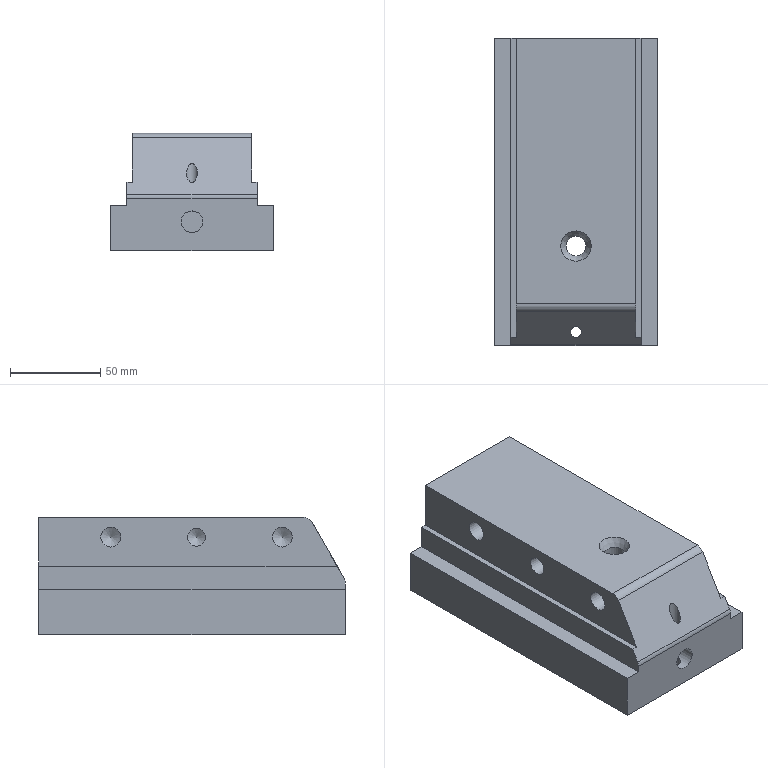Part | NX | features solid 2 | 1 solid | 47 faces | box 90 x 170 x 65 mm | volume 622794 mm3 | plane 25 | cylinder 16 | cone 6 | commonest cylinder face diameters 11 x5 4 x4 10 x3 6 x2 12 x2
STEP:
#1=CARTESIAN_POINT('',(-3.,607.5,-122.196));
#2=VERTEX_POINT('',#1);
#3=CARTESIAN_POINT('',(-2.354,609.851,-122.626));
#4=CARTESIAN_POINT('',(-3.324,607.499,-121.981));
#5=CARTESIAN_POINT('',(-2.352,605.153,-122.625));
#6=CARTESIAN_POINT('',(-0.009342,604.174,-123.187));
#7=CARTESIAN_POINT('',(2.352,605.151,-122.627));
#8=CARTESIAN_POINT('',(3.323,607.488,-121.981));
#9=CARTESIAN_POINT('',(2.356,609.847,-122.624));
#10=CARTESIAN_POINT('',(0.009754,610.826,-123.187));
#11=CARTESIAN_POINT('',(-2.354,609.851,-122.626));
#12=CARTESIAN_POINT('',(-3.324,607.499,-121.981));
#13=CARTESIAN_POINT('',(-2.352,605.153,-122.625));
#14=B_SPLINE_CURVE_WITH_KNOTS('',3,(#3,#4,#5,#6,#7,#8,#9,#10,#11,#12,#13),.UNSPECIFIED.,.T.,.F.,(1,1,1,1,1,1,1,1,1,1,1,1,1,1,1),(-0.00715,-0.004767,-0.002383,0.,0.002383,0.004767,0.00715,0.009533,0.01192,0.0143,0.01668,0.01907,0.02145,0.02383,0.02622),.UNSPECIFIED.);
#15=EDGE_CURVE('',#2,#2,#14,.T.);
#16=ORIENTED_EDGE('',*,*,#15,.T.);
#17=EDGE_LOOP('',(#16));
#18=FACE_BOUND('',#17,.T.);
#19=CARTESIAN_POINT('',(-3.,607.5,-133.));
#20=VERTEX_POINT('',#19);
#21=CARTESIAN_POINT('',(0.,607.5,-133.));
#22=DIRECTION('',(0.,0.,1.));
#23=DIRECTION('',(-1.,0.,0.));
#24=AXIS2_PLACEMENT_3D('',#21,#22,#23);
#25=CIRCLE('',#24,3.);
#26=EDGE_CURVE('',#20,#20,#25,.T.);
#27=ORIENTED_EDGE('',*,*,#26,.F.);
#28=EDGE_LOOP('',(#27));
#29=FACE_BOUND('',#28,.T.);
#30=CARTESIAN_POINT('',(0.,607.5,-133.));
#31=DIRECTION('',(0.,0.,1.));
#32=DIRECTION('',(-1.,0.,0.));
#33=AXIS2_PLACEMENT_3D('',#30,#31,#32);
#34=CYLINDRICAL_SURFACE('',#33,3.);
#35=ADVANCED_FACE('',(#18,#29),#34,.F.);
#36=CARTESIAN_POINT('',(33.,604.619,-95.));
#37=VERTEX_POINT('',#36);
#38=CARTESIAN_POINT('',(33.,770.,-95.));
#39=VERTEX_POINT('',#38);
#40=CARTESIAN_POINT('',(33.,600.,-95.));
#41=DIRECTION('',(0.,1.,0.));
#42=VECTOR('',#41,1000.);
#43=LINE('',#40,#42);
#44=EDGE_CURVE('',#37,#39,#43,.T.);
#45=ORIENTED_EDGE('',*,*,#44,.F.);
#46=CARTESIAN_POINT('',(36.,604.619,-95.));
#47=VERTEX_POINT('',#46);
#48=CARTESIAN_POINT('',(33.,604.619,-95.));
#49=DIRECTION('',(1.,0.,0.));
#50=VECTOR('',#49,1000.);
#51=LINE('',#48,#50);
#52=EDGE_CURVE('',#37,#47,#51,.T.);
#53=ORIENTED_EDGE('',*,*,#52,.T.);
#54=CARTESIAN_POINT('',(36.,770.,-95.));
#55=VERTEX_POINT('',#54);
#56=CARTESIAN_POINT('',(36.,600.,-95.));
#57=DIRECTION('',(0.,1.,0.));
#58=VECTOR('',#57,1000.);
#59=LINE('',#56,#58);
#60=EDGE_CURVE('',#47,#55,#59,.T.);
#61=ORIENTED_EDGE('',*,*,#60,.T.);
#62=CARTESIAN_POINT('',(33.,770.,-95.));
#63=DIRECTION('',(1.,0.,0.));
#64=VECTOR('',#63,1000.);
#65=LINE('',#62,#64);
#66=EDGE_CURVE('',#39,#55,#65,.T.);
#67=ORIENTED_EDGE('',*,*,#66,.F.);
#68=EDGE_LOOP('',(#45,#53,#61,#67));
#69=FACE_BOUND('',#68,.T.);
#70=CARTESIAN_POINT('',(33.,600.,-95.));
#71=DIRECTION('',(0.,0.,1.));
#72=DIRECTION('',(0.,-1.,0.));
#73=AXIS2_PLACEMENT_3D('',#70,#71,#72);
#74=PLANE('',#73);
#75=ADVANCED_FACE('',(#69),#74,.T.);
#76=CARTESIAN_POINT('',(36.,600.67,-101.84));
#77=VERTEX_POINT('',#76);
#78=CARTESIAN_POINT('',(36.,603.464,-97.));
#79=DIRECTION('',(0.,-0.5,-0.866));
#80=VECTOR('',#79,1000.);
#81=LINE('',#78,#80);
#82=EDGE_CURVE('',#47,#77,#81,.T.);
#83=ORIENTED_EDGE('',*,*,#82,.T.);
#84=CARTESIAN_POINT('',(36.,600.,-104.34));
#85=VERTEX_POINT('',#84);
#86=CARTESIAN_POINT('',(36.,605.,-104.34));
#87=DIRECTION('',(1.,0.,0.));
#88=DIRECTION('',(0.,0.,1.));
#89=AXIS2_PLACEMENT_3D('',#86,#87,#88);
#90=CIRCLE('',#89,5.);
#91=EDGE_CURVE('',#77,#85,#90,.T.);
#92=ORIENTED_EDGE('',*,*,#91,.T.);
#93=CARTESIAN_POINT('',(36.,600.,-108.));
#94=VERTEX_POINT('',#93);
#95=CARTESIAN_POINT('',(36.,600.,-95.));
#96=DIRECTION('',(0.,0.,-1.));
#97=VECTOR('',#96,1000.);
#98=LINE('',#95,#97);
#99=EDGE_CURVE('',#85,#94,#98,.T.);
#100=ORIENTED_EDGE('',*,*,#99,.T.);
#101=CARTESIAN_POINT('',(36.,770.,-108.));
#102=VERTEX_POINT('',#101);
#103=CARTESIAN_POINT('',(36.,600.,-108.));
#104=DIRECTION('',(0.,1.,0.));
#105=VECTOR('',#104,1000.);
#106=LINE('',#103,#105);
#107=EDGE_CURVE('',#94,#102,#106,.T.);
#108=ORIENTED_EDGE('',*,*,#107,.T.);
#109=CARTESIAN_POINT('',(36.,770.,-95.));
#110=DIRECTION('',(0.,0.,-1.));
#111=VECTOR('',#110,1000.);
#112=LINE('',#109,#111);
#113=EDGE_CURVE('',#55,#102,#112,.T.);
#114=ORIENTED_EDGE('',*,*,#113,.F.);
#115=ORIENTED_EDGE('',*,*,#60,.F.);
#116=EDGE_LOOP('',(#83,#92,#100,#108,#114,#115));
#117=FACE_BOUND('',#116,.T.);
#118=CARTESIAN_POINT('',(36.,600.,-95.));
#119=DIRECTION('',(1.,0.,0.));
#120=DIRECTION('',(0.,0.,1.));
#121=AXIS2_PLACEMENT_3D('',#118,#119,#120);
#122=PLANE('',#121);
#123=ADVANCED_FACE('',(#117),#122,.T.);
#124=CARTESIAN_POINT('',(45.,770.,-108.));
#125=VERTEX_POINT('',#124);
#126=CARTESIAN_POINT('',(36.,770.,-108.));
#127=DIRECTION('',(1.,0.,0.));
#128=VECTOR('',#127,1000.);
#129=LINE('',#126,#128);
#130=EDGE_CURVE('',#102,#125,#129,.T.);
#131=ORIENTED_EDGE('',*,*,#130,.F.);
#132=ORIENTED_EDGE('',*,*,#107,.F.);
#133=CARTESIAN_POINT('',(45.,600.,-108.));
#134=VERTEX_POINT('',#133);
#135=CARTESIAN_POINT('',(36.,600.,-108.));
#136=DIRECTION('',(1.,0.,0.));
#137=VECTOR('',#136,1000.);
#138=LINE('',#135,#137);
#139=EDGE_CURVE('',#94,#134,#138,.T.);
#140=ORIENTED_EDGE('',*,*,#139,.T.);
#141=CARTESIAN_POINT('',(45.,600.,-108.));
#142=DIRECTION('',(0.,1.,0.));
#143=VECTOR('',#142,1000.);
#144=LINE('',#141,#143);
#145=EDGE_CURVE('',#134,#125,#144,.T.);
#146=ORIENTED_EDGE('',*,*,#145,.T.);
#147=EDGE_LOOP('',(#131,#132,#140,#146));
#148=FACE_BOUND('',#147,.T.);
#149=CARTESIAN_POINT('',(36.,600.,-108.));
#150=DIRECTION('',(0.,0.,1.));
#151=DIRECTION('',(0.,-1.,0.));
#152=AXIS2_PLACEMENT_3D('',#149,#150,#151);
#153=PLANE('',#152);
#154=ADVANCED_FACE('',(#148),#153,.T.);
#155=CARTESIAN_POINT('',(45.,770.,-133.));
#156=VERTEX_POINT('',#155);
#157=CARTESIAN_POINT('',(45.,770.,-108.));
#158=DIRECTION('',(0.,0.,-1.));
#159=VECTOR('',#158,1000.);
#160=LINE('',#157,#159);
#161=EDGE_CURVE('',#125,#156,#160,.T.);
#162=ORIENTED_EDGE('',*,*,#161,.F.);
#163=ORIENTED_EDGE('',*,*,#145,.F.);
#164=CARTESIAN_POINT('',(45.,600.,-133.));
#165=VERTEX_POINT('',#164);
#166=CARTESIAN_POINT('',(45.,600.,-108.));
#167=DIRECTION('',(0.,0.,-1.));
#168=VECTOR('',#167,1000.);
#169=LINE('',#166,#168);
#170=EDGE_CURVE('',#134,#165,#169,.T.);
#171=ORIENTED_EDGE('',*,*,#170,.T.);
#172=CARTESIAN_POINT('',(45.,600.,-133.));
#173=DIRECTION('',(0.,1.,0.));
#174=VECTOR('',#173,1000.);
#175=LINE('',#172,#174);
#176=EDGE_CURVE('',#165,#156,#175,.T.);
#177=ORIENTED_EDGE('',*,*,#176,.T.);
#178=EDGE_LOOP('',(#162,#163,#171,#177));
#179=FACE_BOUND('',#178,.T.);
#180=CARTESIAN_POINT('',(45.,600.,-108.));
#181=DIRECTION('',(1.,0.,0.));
#182=DIRECTION('',(0.,0.,1.));
#183=AXIS2_PLACEMENT_3D('',#180,#181,#182);
#184=PLANE('',#183);
#185=ADVANCED_FACE('',(#179),#184,.T.);
#186=CARTESIAN_POINT('',(18.,615.,-133.));
#187=VERTEX_POINT('',#186);
#188=CARTESIAN_POINT('',(-18.,615.,-133.));
#189=VERTEX_POINT('',#188);
#190=CARTESIAN_POINT('',(20.,615.,-133.));
#191=DIRECTION('',(-1.,0.,0.));
#192=VECTOR('',#191,1000.);
#193=LINE('',#190,#192);
#194=EDGE_CURVE('',#187,#189,#193,.T.);
#195=ORIENTED_EDGE('',*,*,#194,.F.);
#196=CARTESIAN_POINT('',(20.,617.,-133.));
#197=VERTEX_POINT('',#196);
#198=CARTESIAN_POINT('',(18.,617.,-133.));
#199=DIRECTION('',(0.,0.,-1.));
#200=DIRECTION('',(0.,1.,0.));
#201=AXIS2_PLACEMENT_3D('',#198,#199,#200);
#202=CIRCLE('',#201,2.);
#203=EDGE_CURVE('',#187,#197,#202,.F.);
#204=ORIENTED_EDGE('',*,*,#203,.T.);
#205=CARTESIAN_POINT('',(20.,753.,-133.));
#206=VERTEX_POINT('',#205);
#207=CARTESIAN_POINT('',(20.,615.,-133.));
#208=DIRECTION('',(0.,1.,0.));
#209=VECTOR('',#208,1000.);
#210=LINE('',#207,#209);
#211=EDGE_CURVE('',#197,#206,#210,.T.);
#212=ORIENTED_EDGE('',*,*,#211,.T.);
#213=CARTESIAN_POINT('',(18.,755.,-133.));
#214=VERTEX_POINT('',#213);
#215=CARTESIAN_POINT('',(18.,753.,-133.));
#216=DIRECTION('',(0.,0.,-1.));
#217=DIRECTION('',(0.,1.,0.));
#218=AXIS2_PLACEMENT_3D('',#215,#216,#217);
#219=CIRCLE('',#218,2.);
#220=EDGE_CURVE('',#206,#214,#219,.F.);
#221=ORIENTED_EDGE('',*,*,#220,.T.);
#222=CARTESIAN_POINT('',(-18.,755.,-133.));
#223=VERTEX_POINT('',#222);
#224=CARTESIAN_POINT('',(20.,755.,-133.));
#225=DIRECTION('',(-1.,0.,0.));
#226=VECTOR('',#225,1000.);
#227=LINE('',#224,#226);
#228=EDGE_CURVE('',#214,#223,#227,.T.);
#229=ORIENTED_EDGE('',*,*,#228,.T.);
#230=CARTESIAN_POINT('',(-20.,753.,-133.));
#231=VERTEX_POINT('',#230);
#232=CARTESIAN_POINT('',(-18.,753.,-133.));
#233=DIRECTION('',(0.,0.,-1.));
#234=DIRECTION('',(0.,1.,0.));
#235=AXIS2_PLACEMENT_3D('',#232,#233,#234);
#236=CIRCLE('',#235,2.);
#237=EDGE_CURVE('',#223,#231,#236,.F.);
#238=ORIENTED_EDGE('',*,*,#237,.T.);
#239=CARTESIAN_POINT('',(-20.,617.,-133.));
#240=VERTEX_POINT('',#239);
#241=CARTESIAN_POINT('',(-20.,615.,-133.));
#242=DIRECTION('',(0.,1.,0.));
#243=VECTOR('',#242,1000.);
#244=LINE('',#241,#243);
#245=EDGE_CURVE('',#240,#231,#244,.T.);
#246=ORIENTED_EDGE('',*,*,#245,.F.);
#247=CARTESIAN_POINT('',(-18.,617.,-133.));
#248=DIRECTION('',(0.,0.,-1.));
#249=DIRECTION('',(0.,1.,0.));
#250=AXIS2_PLACEMENT_3D('',#247,#248,#249);
#251=CIRCLE('',#250,2.);
#252=EDGE_CURVE('',#240,#189,#251,.F.);
#253=ORIENTED_EDGE('',*,*,#252,.T.);
#254=EDGE_LOOP('',(#195,#204,#212,#221,#229,#238,#246,#253));
#255=FACE_BOUND('',#254,.T.);
#256=ORIENTED_EDGE('',*,*,#26,.T.);
#257=EDGE_LOOP('',(#256));
#258=FACE_BOUND('',#257,.T.);
#259=CARTESIAN_POINT('',(-45.,770.,-133.));
#260=VERTEX_POINT('',#259);
#261=CARTESIAN_POINT('',(45.,770.,-133.));
#262=DIRECTION('',(-1.,0.,0.));
#263=VECTOR('',#262,1000.);
#264=LINE('',#261,#263);
#265=EDGE_CURVE('',#156,#260,#264,.T.);
#266=ORIENTED_EDGE('',*,*,#265,.F.);
#267=ORIENTED_EDGE('',*,*,#176,.F.);
#268=CARTESIAN_POINT('',(-45.,600.,-133.));
#269=VERTEX_POINT('',#268);
#270=CARTESIAN_POINT('',(45.,600.,-133.));
#271=DIRECTION('',(-1.,0.,0.));
#272=VECTOR('',#271,1000.);
#273=LINE('',#270,#272);
#274=EDGE_CURVE('',#165,#269,#273,.T.);
#275=ORIENTED_EDGE('',*,*,#274,.T.);
#276=CARTESIAN_POINT('',(-45.,600.,-133.));
#277=DIRECTION('',(0.,1.,0.));
#278=VECTOR('',#277,1000.);
#279=LINE('',#276,#278);
#280=EDGE_CURVE('',#269,#260,#279,.T.);
#281=ORIENTED_EDGE('',*,*,#280,.T.);
#282=EDGE_LOOP('',(#266,#267,#275,#281));
#283=FACE_BOUND('',#282,.T.);
#284=CARTESIAN_POINT('',(45.,600.,-133.));
#285=DIRECTION('',(0.,0.,-1.));
#286=DIRECTION('',(0.,1.,0.));
#287=AXIS2_PLACEMENT_3D('',#284,#285,#286);
#288=PLANE('',#287);
#289=ADVANCED_FACE('',(#255,#258,#283),#288,.T.);
#290=CARTESIAN_POINT('',(-45.,770.,-108.));
#291=VERTEX_POINT('',#290);
#292=CARTESIAN_POINT('',(-45.,770.,-133.));
#293=DIRECTION('',(0.,0.,1.));
#294=VECTOR('',#293,1000.);
#295=LINE('',#292,#294);
#296=EDGE_CURVE('',#260,#291,#295,.T.);
#297=ORIENTED_EDGE('',*,*,#296,.F.);
#298=ORIENTED_EDGE('',*,*,#280,.F.);
#299=CARTESIAN_POINT('',(-45.,600.,-108.));
#300=VERTEX_POINT('',#299);
#301=CARTESIAN_POINT('',(-45.,600.,-133.));
#302=DIRECTION('',(0.,0.,1.));
#303=VECTOR('',#302,1000.);
#304=LINE('',#301,#303);
#305=EDGE_CURVE('',#269,#300,#304,.T.);
#306=ORIENTED_EDGE('',*,*,#305,.T.);
#307=CARTESIAN_POINT('',(-45.,600.,-108.));
#308=DIRECTION('',(0.,1.,0.));
#309=VECTOR('',#308,1000.);
#310=LINE('',#307,#309);
#311=EDGE_CURVE('',#300,#291,#310,.T.);
#312=ORIENTED_EDGE('',*,*,#311,.T.);
#313=EDGE_LOOP('',(#297,#298,#306,#312));
#314=FACE_BOUND('',#313,.T.);
#315=CARTESIAN_POINT('',(-45.,600.,-133.));
#316=DIRECTION('',(-1.,0.,0.));
#317=DIRECTION('',(0.,0.,-1.));
#318=AXIS2_PLACEMENT_3D('',#315,#316,#317);
#319=PLANE('',#318);
#320=ADVANCED_FACE('',(#314),#319,.T.);
#321=CARTESIAN_POINT('',(-36.,770.,-108.));
#322=VERTEX_POINT('',#321);
#323=CARTESIAN_POINT('',(-45.,770.,-108.));
#324=DIRECTION('',(1.,0.,0.));
#325=VECTOR('',#324,1000.);
#326=LINE('',#323,#325);
#327=EDGE_CURVE('',#291,#322,#326,.T.);
#328=ORIENTED_EDGE('',*,*,#327,.F.);
#329=ORIENTED_EDGE('',*,*,#311,.F.);
#330=CARTESIAN_POINT('',(-36.,600.,-108.));
#331=VERTEX_POINT('',#330);
#332=CARTESIAN_POINT('',(-45.,600.,-108.));
#333=DIRECTION('',(1.,0.,0.));
#334=VECTOR('',#333,1000.);
#335=LINE('',#332,#334);
#336=EDGE_CURVE('',#300,#331,#335,.T.);
#337=ORIENTED_EDGE('',*,*,#336,.T.);
#338=CARTESIAN_POINT('',(-36.,600.,-108.));
#339=DIRECTION('',(0.,1.,0.));
#340=VECTOR('',#339,1000.);
#341=LINE('',#338,#340);
#342=EDGE_CURVE('',#331,#322,#341,.T.);
#343=ORIENTED_EDGE('',*,*,#342,.T.);
#344=EDGE_LOOP('',(#328,#329,#337,#343));
#345=FACE_BOUND('',#344,.T.);
#346=CARTESIAN_POINT('',(-45.,600.,-108.));
#347=DIRECTION('',(0.,0.,1.));
#348=DIRECTION('',(0.,-1.,0.));
#349=AXIS2_PLACEMENT_3D('',#346,#347,#348);
#350=PLANE('',#349);
#351=ADVANCED_FACE('',(#345),#350,.T.);
#352=CARTESIAN_POINT('',(-36.,600.,-104.34));
#353=VERTEX_POINT('',#352);
#354=CARTESIAN_POINT('',(-36.,600.,-108.));
#355=DIRECTION('',(0.,0.,1.));
#356=VECTOR('',#355,1000.);
#357=LINE('',#354,#356);
#358=EDGE_CURVE('',#331,#353,#357,.T.);
#359=ORIENTED_EDGE('',*,*,#358,.T.);
#360=CARTESIAN_POINT('',(-36.,600.67,-101.84));
#361=VERTEX_POINT('',#360);
#362=CARTESIAN_POINT('',(-36.,605.,-104.34));
#363=DIRECTION('',(-1.,0.,0.));
#364=DIRECTION('',(0.,0.,-1.));
#365=AXIS2_PLACEMENT_3D('',#362,#363,#364);
#366=CIRCLE('',#365,5.);
#367=EDGE_CURVE('',#353,#361,#366,.T.);
#368=ORIENTED_EDGE('',*,*,#367,.T.);
#369=CARTESIAN_POINT('',(-36.,604.619,-95.));
#370=VERTEX_POINT('',#369);
#371=CARTESIAN_POINT('',(-36.,597.835,-106.75));
#372=DIRECTION('',(0.,0.5,0.866));
#373=VECTOR('',#372,1000.);
#374=LINE('',#371,#373);
#375=EDGE_CURVE('',#361,#370,#374,.T.);
#376=ORIENTED_EDGE('',*,*,#375,.T.);
#377=CARTESIAN_POINT('',(-36.,770.,-95.));
#378=VERTEX_POINT('',#377);
#379=CARTESIAN_POINT('',(-36.,600.,-95.));
#380=DIRECTION('',(0.,1.,0.));
#381=VECTOR('',#380,1000.);
#382=LINE('',#379,#381);
#383=EDGE_CURVE('',#370,#378,#382,.T.);
#384=ORIENTED_EDGE('',*,*,#383,.T.);
#385=CARTESIAN_POINT('',(-36.,770.,-108.));
#386=DIRECTION('',(0.,0.,1.));
#387=VECTOR('',#386,1000.);
#388=LINE('',#385,#387);
#389=EDGE_CURVE('',#322,#378,#388,.T.);
#390=ORIENTED_EDGE('',*,*,#389,.F.);
#391=ORIENTED_EDGE('',*,*,#342,.F.);
#392=EDGE_LOOP('',(#359,#368,#376,#384,#390,#391));
#393=FACE_BOUND('',#392,.T.);
#394=CARTESIAN_POINT('',(-36.,600.,-108.));
#395=DIRECTION('',(-1.,0.,0.));
#396=DIRECTION('',(0.,0.,-1.));
#397=AXIS2_PLACEMENT_3D('',#394,#395,#396);
#398=PLANE('',#397);
#399=ADVANCED_FACE('',(#393),#398,.T.);
#400=ORIENTED_EDGE('',*,*,#383,.F.);
#401=CARTESIAN_POINT('',(-33.,604.619,-95.));
#402=VERTEX_POINT('',#401);
#403=CARTESIAN_POINT('',(-33.,604.619,-95.));
#404=DIRECTION('',(1.,0.,0.));
#405=VECTOR('',#404,1000.);
#406=LINE('',#403,#405);
#407=EDGE_CURVE('',#370,#402,#406,.T.);
#408=ORIENTED_EDGE('',*,*,#407,.T.);
#409=CARTESIAN_POINT('',(-33.,770.,-95.));
#410=VERTEX_POINT('',#409);
#411=CARTESIAN_POINT('',(-33.,600.,-95.));
#412=DIRECTION('',(0.,1.,0.));
#413=VECTOR('',#412,1000.);
#414=LINE('',#411,#413);
#415=EDGE_CURVE('',#402,#410,#414,.T.);
#416=ORIENTED_EDGE('',*,*,#415,.T.);
#417=CARTESIAN_POINT('',(-33.,770.,-95.));
#418=DIRECTION('',(-1.,0.,0.));
#419=VECTOR('',#418,1000.);
#420=LINE('',#417,#419);
#421=EDGE_CURVE('',#410,#378,#420,.T.);
#422=ORIENTED_EDGE('',*,*,#421,.T.);
#423=EDGE_LOOP('',(#400,#408,#416,#422));
#424=FACE_BOUND('',#423,.T.);
#425=CARTESIAN_POINT('',(-33.,600.,-95.));
#426=DIRECTION('',(0.,0.,-1.));
#427=DIRECTION('',(0.,1.,0.));
#428=AXIS2_PLACEMENT_3D('',#425,#426,#427);
#429=PLANE('',#428);
#430=ADVANCED_FACE('',(#424),#429,.F.);
#431=CARTESIAN_POINT('',(-33.,635.,-73.5));
#432=VERTEX_POINT('',#431);
#433=CARTESIAN_POINT('',(-33.,635.,-79.));
#434=DIRECTION('',(1.,0.,0.));
#435=DIRECTION('',(0.,0.,1.));
#436=AXIS2_PLACEMENT_3D('',#433,#434,#435);
#437=CIRCLE('',#436,5.5);
#438=EDGE_CURVE('',#432,#432,#437,.T.);
#439=ORIENTED_EDGE('',*,*,#438,.T.);
#440=EDGE_LOOP('',(#439));
#441=FACE_BOUND('',#440,.T.);
#442=CARTESIAN_POINT('',(-33.,682.5,-74.));
#443=VERTEX_POINT('',#442);
#444=CARTESIAN_POINT('',(-33.,682.5,-79.));
#445=DIRECTION('',(1.,0.,0.));
#446=DIRECTION('',(0.,0.,1.));
#447=AXIS2_PLACEMENT_3D('',#444,#445,#446);
#448=CIRCLE('',#447,5.);
#449=EDGE_CURVE('',#443,#443,#448,.T.);
#450=ORIENTED_EDGE('',*,*,#449,.T.);
#451=EDGE_LOOP('',(#450));
#452=FACE_BOUND('',#451,.T.);
#453=CARTESIAN_POINT('',(-33.,730.,-73.5));
#454=VERTEX_POINT('',#453);
#455=CARTESIAN_POINT('',(-33.,730.,-79.));
#456=DIRECTION('',(1.,0.,0.));
#457=DIRECTION('',(0.,0.,1.));
#458=AXIS2_PLACEMENT_3D('',#455,#456,#457);
#459=CIRCLE('',#458,5.5);
#460=EDGE_CURVE('',#454,#454,#459,.T.);
#461=ORIENTED_EDGE('',*,*,#460,.T.);
#462=EDGE_LOOP('',(#461));
#463=FACE_BOUND('',#462,.T.);
#464=CARTESIAN_POINT('',(-33.,618.764,-70.5));
#465=VERTEX_POINT('',#464);
#466=CARTESIAN_POINT('',(-33.,620.207,-68.));
#467=DIRECTION('',(0.,0.5,0.866));
#468=VECTOR('',#467,1000.);
#469=LINE('',#466,#468);
#470=EDGE_CURVE('',#402,#465,#469,.T.);
#471=ORIENTED_EDGE('',*,*,#470,.T.);
#472=CARTESIAN_POINT('',(-33.,623.094,-68.));
#473=VERTEX_POINT('',#472);
#474=CARTESIAN_POINT('',(-33.,623.094,-73.));
#475=DIRECTION('',(1.,0.,0.));
#476=DIRECTION('',(0.,0.,1.));
#477=AXIS2_PLACEMENT_3D('',#474,#475,#476);
#478=CIRCLE('',#477,5.);
#479=EDGE_CURVE('',#465,#473,#478,.F.);
#480=ORIENTED_EDGE('',*,*,#479,.T.);
#481=CARTESIAN_POINT('',(-33.,770.,-68.));
#482=VERTEX_POINT('',#481);
#483=CARTESIAN_POINT('',(-33.,600.,-68.));
#484=DIRECTION('',(0.,1.,0.));
#485=VECTOR('',#484,1000.);
#486=LINE('',#483,#485);
#487=EDGE_CURVE('',#473,#482,#486,.T.);
#488=ORIENTED_EDGE('',*,*,#487,.T.);
#489=CARTESIAN_POINT('',(-33.,770.,-68.));
#490=DIRECTION('',(0.,0.,-1.));
#491=VECTOR('',#490,1000.);
#492=LINE('',#489,#491);
#493=EDGE_CURVE('',#482,#410,#492,.T.);
#494=ORIENTED_EDGE('',*,*,#493,.T.);
#495=ORIENTED_EDGE('',*,*,#415,.F.);
#496=EDGE_LOOP('',(#471,#480,#488,#494,#495));
#497=FACE_BOUND('',#496,.T.);
#498=CARTESIAN_POINT('',(-33.,600.,-68.));
#499=DIRECTION('',(1.,0.,0.));
#500=DIRECTION('',(0.,0.,1.));
#501=AXIS2_PLACEMENT_3D('',#498,#499,#500);
#502=PLANE('',#501);
#503=ADVANCED_FACE('',(#441,#452,#463,#497),#502,.F.);
#504=CARTESIAN_POINT('',(0.,646.613,-68.));
#505=VERTEX_POINT('',#504);
#506=CARTESIAN_POINT('',(0.,655.,-68.));
#507=DIRECTION('',(0.,0.,1.));
#508=DIRECTION('',(0.,-1.,0.));
#509=AXIS2_PLACEMENT_3D('',#506,#507,#508);
#510=CIRCLE('',#509,8.387);
#511=EDGE_CURVE('',#505,#505,#510,.F.);
#512=ORIENTED_EDGE('',*,*,#511,.T.);
#513=EDGE_LOOP('',(#512));
#514=FACE_BOUND('',#513,.T.);
#515=ORIENTED_EDGE('',*,*,#487,.F.);
#516=CARTESIAN_POINT('',(33.,623.094,-68.));
#517=VERTEX_POINT('',#516);
#518=CARTESIAN_POINT('',(-33.,623.094,-68.));
#519=DIRECTION('',(1.,0.,0.));
#520=VECTOR('',#519,1000.);
#521=LINE('',#518,#520);
#522=EDGE_CURVE('',#473,#517,#521,.T.);
#523=ORIENTED_EDGE('',*,*,#522,.T.);
#524=CARTESIAN_POINT('',(33.,770.,-68.));
#525=VERTEX_POINT('',#524);
#526=CARTESIAN_POINT('',(33.,600.,-68.));
#527=DIRECTION('',(0.,1.,0.));
#528=VECTOR('',#527,1000.);
#529=LINE('',#526,#528);
#530=EDGE_CURVE('',#517,#525,#529,.T.);
#531=ORIENTED_EDGE('',*,*,#530,.T.);
#532=CARTESIAN_POINT('',(-33.,770.,-68.));
#533=DIRECTION('',(1.,0.,0.));
#534=VECTOR('',#533,1000.);
#535=LINE('',#532,#534);
#536=EDGE_CURVE('',#482,#525,#535,.T.);
#537=ORIENTED_EDGE('',*,*,#536,.F.);
#538=EDGE_LOOP('',(#515,#523,#531,#537));
#539=FACE_BOUND('',#538,.T.);
#540=CARTESIAN_POINT('',(-33.,600.,-68.));
#541=DIRECTION('',(0.,0.,1.));
#542=DIRECTION('',(0.,-1.,0.));
#543=AXIS2_PLACEMENT_3D('',#540,#541,#542);
#544=PLANE('',#543);
#545=ADVANCED_FACE('',(#514,#539),#544,.T.);
#546=CARTESIAN_POINT('',(33.,635.,-73.5));
#547=VERTEX_POINT('',#546);
#548=CARTESIAN_POINT('',(33.,635.,-79.));
#549=DIRECTION('',(-1.,0.,0.));
#550=DIRECTION('',(0.,0.,1.));
#551=AXIS2_PLACEMENT_3D('',#548,#549,#550);
#552=CIRCLE('',#551,5.5);
#553=EDGE_CURVE('',#547,#547,#552,.T.);
#554=ORIENTED_EDGE('',*,*,#553,.T.);
#555=EDGE_LOOP('',(#554));
#556=FACE_BOUND('',#555,.T.);
#557=CARTESIAN_POINT('',(33.,730.,-73.5));
#558=VERTEX_POINT('',#557);
#559=CARTESIAN_POINT('',(33.,730.,-79.));
#560=DIRECTION('',(1.,0.,0.));
#561=DIRECTION('',(0.,0.,1.));
#562=AXIS2_PLACEMENT_3D('',#559,#560,#561);
#563=CIRCLE('',#562,5.5);
#564=EDGE_CURVE('',#558,#558,#563,.T.);
#565=ORIENTED_EDGE('',*,*,#564,.F.);
#566=EDGE_LOOP('',(#565));
#567=FACE_BOUND('',#566,.T.);
#568=ORIENTED_EDGE('',*,*,#530,.F.);
#569=CARTESIAN_POINT('',(33.,618.764,-70.5));
#570=VERTEX_POINT('',#569);
#571=CARTESIAN_POINT('',(33.,623.094,-73.));
#572=DIRECTION('',(1.,0.,0.));
#573=DIRECTION('',(0.,0.,1.));
#574=AXIS2_PLACEMENT_3D('',#571,#572,#573);
#575=CIRCLE('',#574,5.);
#576=EDGE_CURVE('',#517,#570,#575,.T.);
#577=ORIENTED_EDGE('',*,*,#576,.T.);
#578=CARTESIAN_POINT('',(33.,615.155,-76.75));
#579=DIRECTION('',(0.,-0.5,-0.866));
#580=VECTOR('',#579,1000.);
#581=LINE('',#578,#580);
#582=EDGE_CURVE('',#570,#37,#581,.T.);
#583=ORIENTED_EDGE('',*,*,#582,.T.);
#584=ORIENTED_EDGE('',*,*,#44,.T.);
#585=CARTESIAN_POINT('',(33.,770.,-68.));
#586=DIRECTION('',(0.,0.,-1.));
#587=VECTOR('',#586,1000.);
#588=LINE('',#585,#587);
#589=EDGE_CURVE('',#525,#39,#588,.T.);
#590=ORIENTED_EDGE('',*,*,#589,.F.);
#591=EDGE_LOOP('',(#568,#577,#583,#584,#590));
#592=FACE_BOUND('',#591,.T.);
#593=CARTESIAN_POINT('',(33.,600.,-68.));
#594=DIRECTION('',(1.,0.,0.));
#595=DIRECTION('',(0.,0.,1.));
#596=AXIS2_PLACEMENT_3D('',#593,#594,#595);
#597=PLANE('',#596);
#598=ADVANCED_FACE('',(#556,#567,#592),#597,.T.);
#599=CARTESIAN_POINT('',(0.,600.,-123.));
#600=VERTEX_POINT('',#599);
#601=CARTESIAN_POINT('',(0.,600.,-117.));
#602=DIRECTION('',(0.,1.,0.));
#603=DIRECTION('',(0.,0.,-1.));
#604=AXIS2_PLACEMENT_3D('',#601,#602,#603);
#605=CIRCLE('',#604,6.);
#606=EDGE_CURVE('',#600,#600,#605,.T.);
#607=ORIENTED_EDGE('',*,*,#606,.T.);
#608=EDGE_LOOP('',(#607));
#609=FACE_BOUND('',#608,.T.);
#610=ORIENTED_EDGE('',*,*,#99,.F.);
#611=CARTESIAN_POINT('',(-36.,600.,-104.34));
#612=DIRECTION('',(-1.,0.,0.));
#613=VECTOR('',#612,1000.);
#614=LINE('',#611,#613);
#615=EDGE_CURVE('',#85,#353,#614,.T.);
#616=ORIENTED_EDGE('',*,*,#615,.T.);
#617=ORIENTED_EDGE('',*,*,#358,.F.);
#618=ORIENTED_EDGE('',*,*,#336,.F.);
#619=ORIENTED_EDGE('',*,*,#305,.F.);
#620=ORIENTED_EDGE('',*,*,#274,.F.);
#621=ORIENTED_EDGE('',*,*,#170,.F.);
#622=ORIENTED_EDGE('',*,*,#139,.F.);
#623=EDGE_LOOP('',(#610,#616,#617,#618,#619,#620,#621,#622));
#624=FACE_BOUND('',#623,.T.);
#625=CARTESIAN_POINT('',(36.,600.,-95.));
#626=DIRECTION('',(0.,1.,0.));
#627=DIRECTION('',(0.,0.,1.));
#628=AXIS2_PLACEMENT_3D('',#625,#626,#627);
#629=PLANE('',#628);
#630=ADVANCED_FACE('',(#609,#624),#629,.F.);
#631=ORIENTED_EDGE('',*,*,#66,.T.);
#632=ORIENTED_EDGE('',*,*,#113,.T.);
#633=ORIENTED_EDGE('',*,*,#130,.T.);
#634=ORIENTED_EDGE('',*,*,#161,.T.);
#635=ORIENTED_EDGE('',*,*,#265,.T.);
#636=ORIENTED_EDGE('',*,*,#296,.T.);
#637=ORIENTED_EDGE('',*,*,#327,.T.);
#638=ORIENTED_EDGE('',*,*,#389,.T.);
#639=ORIENTED_EDGE('',*,*,#421,.F.);
#640=ORIENTED_EDGE('',*,*,#493,.F.);
#641=ORIENTED_EDGE('',*,*,#536,.T.);
#642=ORIENTED_EDGE('',*,*,#589,.T.);
#643=EDGE_LOOP('',(#631,#632,#633,#634,#635,#636,#637,#638,#639,#640,#641,#642));
#644=FACE_BOUND('',#643,.T.);
#645=CARTESIAN_POINT('',(36.,770.,-95.));
#646=DIRECTION('',(0.,1.,0.));
#647=DIRECTION('',(0.,0.,1.));
#648=AXIS2_PLACEMENT_3D('',#645,#646,#647);
#649=PLANE('',#648);
#650=ADVANCED_FACE('',(#644),#649,.T.);
#651=CARTESIAN_POINT('',(0.,610.5,-84.813));
#652=VERTEX_POINT('',#651);
#653=CARTESIAN_POINT('',(0.,607.5,-90.01));
#654=DIRECTION('',(0.,-0.866,0.5));
#655=DIRECTION('',(0.,0.5,0.866));
#656=AXIS2_PLACEMENT_3D('',#653,#654,#655);
#657=ELLIPSE('',#656,6.,3.);
#658=EDGE_CURVE('',#652,#652,#657,.T.);
#659=ORIENTED_EDGE('',*,*,#658,.F.);
#660=EDGE_LOOP('',(#659));
#661=FACE_BOUND('',#660,.T.);
#662=ORIENTED_EDGE('',*,*,#375,.F.);
#663=CARTESIAN_POINT('',(36.,600.67,-101.84));
#664=DIRECTION('',(-1.,0.,0.));
#665=VECTOR('',#664,1000.);
#666=LINE('',#663,#665);
#667=EDGE_CURVE('',#361,#77,#666,.F.);
#668=ORIENTED_EDGE('',*,*,#667,.T.);
#669=ORIENTED_EDGE('',*,*,#82,.F.);
#670=ORIENTED_EDGE('',*,*,#52,.F.);
#671=ORIENTED_EDGE('',*,*,#582,.F.);
#672=CARTESIAN_POINT('',(-33.,618.764,-70.5));
#673=DIRECTION('',(1.,0.,0.));
#674=VECTOR('',#673,1000.);
#675=LINE('',#672,#674);
#676=EDGE_CURVE('',#570,#465,#675,.F.);
#677=ORIENTED_EDGE('',*,*,#676,.T.);
#678=ORIENTED_EDGE('',*,*,#470,.F.);
#679=ORIENTED_EDGE('',*,*,#407,.F.);
#680=EDGE_LOOP('',(#662,#668,#669,#670,#671,#677,#678,#679));
#681=FACE_BOUND('',#680,.T.);
#682=CARTESIAN_POINT('',(-33.,620.207,-68.));
#683=DIRECTION('',(0.,-0.866,0.5));
#684=DIRECTION('',(0.,-0.5,-0.866));
#685=AXIS2_PLACEMENT_3D('',#682,#683,#684);
#686=PLANE('',#685);
#687=ADVANCED_FACE('',(#661,#681),#686,.T.);
#688=CARTESIAN_POINT('',(-3.,607.5,-111.804));
#689=VERTEX_POINT('',#688);
#690=CARTESIAN_POINT('',(-2.354,605.149,-111.374));
#691=CARTESIAN_POINT('',(-3.324,607.501,-112.019));
#692=CARTESIAN_POINT('',(-2.352,609.847,-111.375));
#693=CARTESIAN_POINT('',(-0.009342,610.826,-110.813));
#694=CARTESIAN_POINT('',(2.352,609.849,-111.373));
#695=CARTESIAN_POINT('',(3.323,607.512,-112.019));
#696=CARTESIAN_POINT('',(2.356,605.153,-111.376));
#697=CARTESIAN_POINT('',(0.009754,604.174,-110.813));
#698=CARTESIAN_POINT('',(-2.354,605.149,-111.374));
#699=CARTESIAN_POINT('',(-3.324,607.501,-112.019));
#700=CARTESIAN_POINT('',(-2.352,609.847,-111.375));
#701=B_SPLINE_CURVE_WITH_KNOTS('',3,(#690,#691,#692,#693,#694,#695,#696,#697,#698,#699,#700),.UNSPECIFIED.,.T.,.F.,(1,1,1,1,1,1,1,1,1,1,1,1,1,1,1),(-0.00715,-0.004767,-0.002383,0.,0.002383,0.004767,0.00715,0.009533,0.01192,0.0143,0.01668,0.01907,0.02145,0.02383,0.02622),.UNSPECIFIED.);
#702=EDGE_CURVE('',#689,#689,#701,.T.);
#703=ORIENTED_EDGE('',*,*,#702,.T.);
#704=EDGE_LOOP('',(#703));
#705=FACE_BOUND('',#704,.T.);
#706=ORIENTED_EDGE('',*,*,#658,.T.);
#707=EDGE_LOOP('',(#706));
#708=FACE_BOUND('',#707,.T.);
#709=CARTESIAN_POINT('',(0.,607.5,-133.));
#710=DIRECTION('',(0.,0.,1.));
#711=DIRECTION('',(-1.,0.,0.));
#712=AXIS2_PLACEMENT_3D('',#709,#710,#711);
#713=CYLINDRICAL_SURFACE('',#712,3.);
#714=ADVANCED_FACE('',(#705,#708),#713,.F.);
#715=CARTESIAN_POINT('',(0.,615.,-123.));
#716=VERTEX_POINT('',#715);
#717=CARTESIAN_POINT('',(0.,615.,-117.));
#718=DIRECTION('',(0.,-1.,0.));
#719=DIRECTION('',(0.,0.,-1.));
#720=AXIS2_PLACEMENT_3D('',#717,#718,#719);
#721=CIRCLE('',#720,6.);
#722=EDGE_CURVE('',#716,#716,#721,.T.);
#723=ORIENTED_EDGE('',*,*,#722,.T.);
#724=EDGE_LOOP('',(#723));
#725=FACE_BOUND('',#724,.T.);
#726=CARTESIAN_POINT('',(-18.,615.,-103.));
#727=VERTEX_POINT('',#726);
#728=CARTESIAN_POINT('',(18.,615.,-103.));
#729=VERTEX_POINT('',#728);
#730=CARTESIAN_POINT('',(20.,615.,-103.));
#731=DIRECTION('',(1.,0.,0.));
#732=VECTOR('',#731,1000.);
#733=LINE('',#730,#732);
#734=EDGE_CURVE('',#727,#729,#733,.T.);
#735=ORIENTED_EDGE('',*,*,#734,.T.);
#736=CARTESIAN_POINT('',(18.,615.,-133.));
#737=DIRECTION('',(0.,0.,1.));
#738=VECTOR('',#737,1000.);
#739=LINE('',#736,#738);
#740=EDGE_CURVE('',#729,#187,#739,.F.);
#741=ORIENTED_EDGE('',*,*,#740,.T.);
#742=ORIENTED_EDGE('',*,*,#194,.T.);
#743=CARTESIAN_POINT('',(-18.,615.,-103.));
#744=DIRECTION('',(0.,0.,1.));
#745=VECTOR('',#744,1000.);
#746=LINE('',#743,#745);
#747=EDGE_CURVE('',#189,#727,#746,.T.);
#748=ORIENTED_EDGE('',*,*,#747,.T.);
#749=EDGE_LOOP('',(#735,#741,#742,#748));
#750=FACE_BOUND('',#749,.T.);
#751=CARTESIAN_POINT('',(20.,615.,-133.));
#752=DIRECTION('',(0.,-1.,0.));
#753=DIRECTION('',(0.,0.,1.));
#754=AXIS2_PLACEMENT_3D('',#751,#752,#753);
#755=PLANE('',#754);
#756=ADVANCED_FACE('',(#725,#750),#755,.F.);
#757=ORIENTED_EDGE('',*,*,#245,.T.);
#758=CARTESIAN_POINT('',(-20.,753.,-103.));
#759=VERTEX_POINT('',#758);
#760=CARTESIAN_POINT('',(-20.,753.,-103.));
#761=DIRECTION('',(0.,0.,1.));
#762=VECTOR('',#761,1000.);
#763=LINE('',#760,#762);
#764=EDGE_CURVE('',#231,#759,#763,.T.);
#765=ORIENTED_EDGE('',*,*,#764,.T.);
#766=CARTESIAN_POINT('',(-20.,617.,-103.));
#767=VERTEX_POINT('',#766);
#768=CARTESIAN_POINT('',(-20.,615.,-103.));
#769=DIRECTION('',(0.,-1.,0.));
#770=VECTOR('',#769,1000.);
#771=LINE('',#768,#770);
#772=EDGE_CURVE('',#759,#767,#771,.T.);
#773=ORIENTED_EDGE('',*,*,#772,.T.);
#774=CARTESIAN_POINT('',(-20.,617.,-133.));
#775=DIRECTION('',(0.,0.,1.));
#776=VECTOR('',#775,1000.);
#777=LINE('',#774,#776);
#778=EDGE_CURVE('',#767,#240,#777,.F.);
#779=ORIENTED_EDGE('',*,*,#778,.T.);
#780=EDGE_LOOP('',(#757,#765,#773,#779));
#781=FACE_BOUND('',#780,.T.);
#782=CARTESIAN_POINT('',(-20.,615.,-133.));
#783=DIRECTION('',(-1.,0.,0.));
#784=DIRECTION('',(0.,0.,-1.));
#785=AXIS2_PLACEMENT_3D('',#782,#783,#784);
#786=PLANE('',#785);
#787=ADVANCED_FACE('',(#781),#786,.F.);
#788=CARTESIAN_POINT('',(0.,755.,-111.));
#789=VERTEX_POINT('',#788);
#790=CARTESIAN_POINT('',(0.,755.,-117.));
#791=DIRECTION('',(0.,1.,0.));
#792=DIRECTION('',(0.,0.,1.));
#793=AXIS2_PLACEMENT_3D('',#790,#791,#792);
#794=CIRCLE('',#793,6.);
#795=EDGE_CURVE('',#789,#789,#794,.T.);
#796=ORIENTED_EDGE('',*,*,#795,.T.);
#797=EDGE_LOOP('',(#796));
#798=FACE_BOUND('',#797,.T.);
#799=ORIENTED_EDGE('',*,*,#228,.F.);
#800=CARTESIAN_POINT('',(18.,755.,-103.));
#801=VERTEX_POINT('',#800);
#802=CARTESIAN_POINT('',(18.,755.,-103.));
#803=DIRECTION('',(0.,0.,1.));
#804=VECTOR('',#803,1000.);
#805=LINE('',#802,#804);
#806=EDGE_CURVE('',#214,#801,#805,.T.);
#807=ORIENTED_EDGE('',*,*,#806,.T.);
#808=CARTESIAN_POINT('',(-18.,755.,-103.));
#809=VERTEX_POINT('',#808);
#810=CARTESIAN_POINT('',(-20.,755.,-103.));
#811=DIRECTION('',(-1.,0.,0.));
#812=VECTOR('',#811,1000.);
#813=LINE('',#810,#812);
#814=EDGE_CURVE('',#801,#809,#813,.T.);
#815=ORIENTED_EDGE('',*,*,#814,.T.);
#816=CARTESIAN_POINT('',(-18.,755.,-133.));
#817=DIRECTION('',(0.,0.,1.));
#818=VECTOR('',#817,1000.);
#819=LINE('',#816,#818);
#820=EDGE_CURVE('',#809,#223,#819,.F.);
#821=ORIENTED_EDGE('',*,*,#820,.T.);
#822=EDGE_LOOP('',(#799,#807,#815,#821));
#823=FACE_BOUND('',#822,.T.);
#824=CARTESIAN_POINT('',(-20.,755.,-133.));
#825=DIRECTION('',(0.,1.,0.));
#826=DIRECTION('',(0.,0.,-1.));
#827=AXIS2_PLACEMENT_3D('',#824,#825,#826);
#828=PLANE('',#827);
#829=ADVANCED_FACE('',(#798,#823),#828,.F.);
#830=CARTESIAN_POINT('',(-18.,753.,-101.));
#831=VERTEX_POINT('',#830);
#832=CARTESIAN_POINT('',(18.,753.,-101.));
#833=VERTEX_POINT('',#832);
#834=CARTESIAN_POINT('',(20.,753.,-101.));
#835=DIRECTION('',(1.,0.,0.));
#836=VECTOR('',#835,1000.);
#837=LINE('',#834,#836);
#838=EDGE_CURVE('',#831,#833,#837,.T.);
#839=ORIENTED_EDGE('',*,*,#838,.T.);
#840=CARTESIAN_POINT('',(18.,617.,-101.));
#841=VERTEX_POINT('',#840);
#842=CARTESIAN_POINT('',(18.,615.,-101.));
#843=DIRECTION('',(0.,-1.,0.));
#844=VECTOR('',#843,1000.);
#845=LINE('',#842,#844);
#846=EDGE_CURVE('',#833,#841,#845,.T.);
#847=ORIENTED_EDGE('',*,*,#846,.T.);
#848=CARTESIAN_POINT('',(-18.,617.,-101.));
#849=VERTEX_POINT('',#848);
#850=CARTESIAN_POINT('',(-20.,617.,-101.));
#851=DIRECTION('',(-1.,0.,0.));
#852=VECTOR('',#851,1000.);
#853=LINE('',#850,#852);
#854=EDGE_CURVE('',#841,#849,#853,.T.);
#855=ORIENTED_EDGE('',*,*,#854,.T.);
#856=CARTESIAN_POINT('',(-18.,755.,-101.));
#857=DIRECTION('',(0.,1.,0.));
#858=VECTOR('',#857,1000.);
#859=LINE('',#856,#858);
#860=EDGE_CURVE('',#849,#831,#859,.T.);
#861=ORIENTED_EDGE('',*,*,#860,.T.);
#862=EDGE_LOOP('',(#839,#847,#855,#861));
#863=FACE_BOUND('',#862,.T.);
#864=CARTESIAN_POINT('',(0.,649.5,-101.));
#865=VERTEX_POINT('',#864);
#866=CARTESIAN_POINT('',(0.,655.,-101.));
#867=DIRECTION('',(0.,0.,1.));
#868=DIRECTION('',(0.,-1.,0.));
#869=AXIS2_PLACEMENT_3D('',#866,#867,#868);
#870=CIRCLE('',#869,5.5);
#871=EDGE_CURVE('',#865,#865,#870,.T.);
#872=ORIENTED_EDGE('',*,*,#871,.T.);
#873=EDGE_LOOP('',(#872));
#874=FACE_BOUND('',#873,.T.);
#875=CARTESIAN_POINT('',(20.,615.,-101.));
#876=DIRECTION('',(0.,0.,1.));
#877=DIRECTION('',(-1.,0.,0.));
#878=AXIS2_PLACEMENT_3D('',#875,#876,#877);
#879=PLANE('',#878);
#880=ADVANCED_FACE('',(#863,#874),#879,.F.);
#881=ORIENTED_EDGE('',*,*,#211,.F.);
#882=CARTESIAN_POINT('',(20.,617.,-103.));
#883=VERTEX_POINT('',#882);
#884=CARTESIAN_POINT('',(20.,617.,-103.));
#885=DIRECTION('',(0.,0.,1.));
#886=VECTOR('',#885,1000.);
#887=LINE('',#884,#886);
#888=EDGE_CURVE('',#197,#883,#887,.T.);
#889=ORIENTED_EDGE('',*,*,#888,.T.);
#890=CARTESIAN_POINT('',(20.,753.,-103.));
#891=VERTEX_POINT('',#890);
#892=CARTESIAN_POINT('',(20.,755.,-103.));
#893=DIRECTION('',(0.,1.,0.));
#894=VECTOR('',#893,1000.);
#895=LINE('',#892,#894);
#896=EDGE_CURVE('',#883,#891,#895,.T.);
#897=ORIENTED_EDGE('',*,*,#896,.T.);
#898=CARTESIAN_POINT('',(20.,753.,-133.));
#899=DIRECTION('',(0.,0.,1.));
#900=VECTOR('',#899,1000.);
#901=LINE('',#898,#900);
#902=EDGE_CURVE('',#891,#206,#901,.F.);
#903=ORIENTED_EDGE('',*,*,#902,.T.);
#904=EDGE_LOOP('',(#881,#889,#897,#903));
#905=FACE_BOUND('',#904,.T.);
#906=CARTESIAN_POINT('',(20.,755.,-133.));
#907=DIRECTION('',(1.,0.,0.));
#908=DIRECTION('',(0.,0.,1.));
#909=AXIS2_PLACEMENT_3D('',#906,#907,#908);
#910=PLANE('',#909);
#911=ADVANCED_FACE('',(#905),#910,.F.);
#912=CARTESIAN_POINT('',(0.,759.,-123.));
#913=VERTEX_POINT('',#912);
#914=CARTESIAN_POINT('',(0.,759.,-117.));
#915=DIRECTION('',(0.,1.,0.));
#916=DIRECTION('',(0.,0.,-1.));
#917=AXIS2_PLACEMENT_3D('',#914,#915,#916);
#918=CIRCLE('',#917,6.);
#919=EDGE_CURVE('',#913,#913,#918,.T.);
#920=ORIENTED_EDGE('',*,*,#919,.F.);
#921=EDGE_LOOP('',(#920));
#922=FACE_BOUND('',#921,.T.);
#923=CARTESIAN_POINT('',(0.,759.,-117.));
#924=DIRECTION('',(0.,1.,0.));
#925=DIRECTION('',(0.,0.,-1.));
#926=AXIS2_PLACEMENT_3D('',#923,#924,#925);
#927=PLANE('',#926);
#928=ADVANCED_FACE('',(#922),#927,.F.);
#929=ORIENTED_EDGE('',*,*,#919,.T.);
#930=EDGE_LOOP('',(#929));
#931=FACE_BOUND('',#930,.T.);
#932=ORIENTED_EDGE('',*,*,#795,.F.);
#933=EDGE_LOOP('',(#932));
#934=FACE_BOUND('',#933,.T.);
#935=CARTESIAN_POINT('',(0.,600.,-117.));
#936=DIRECTION('',(0.,1.,0.));
#937=DIRECTION('',(0.,0.,-1.));
#938=AXIS2_PLACEMENT_3D('',#935,#936,#937);
#939=CYLINDRICAL_SURFACE('',#938,6.);
#940=ADVANCED_FACE('',(#931,#934),#939,.F.);
#941=ORIENTED_EDGE('',*,*,#702,.F.);
#942=EDGE_LOOP('',(#941));
#943=FACE_BOUND('',#942,.T.);
#944=ORIENTED_EDGE('',*,*,#606,.F.);
#945=EDGE_LOOP('',(#944));
#946=FACE_BOUND('',#945,.T.);
#947=ORIENTED_EDGE('',*,*,#722,.F.);
#948=EDGE_LOOP('',(#947));
#949=FACE_BOUND('',#948,.T.);
#950=ORIENTED_EDGE('',*,*,#15,.F.);
#951=EDGE_LOOP('',(#950));
#952=FACE_BOUND('',#951,.T.);
#953=CARTESIAN_POINT('',(0.,600.,-117.));
#954=DIRECTION('',(0.,1.,0.));
#955=DIRECTION('',(0.,0.,-1.));
#956=AXIS2_PLACEMENT_3D('',#953,#954,#955);
#957=CYLINDRICAL_SURFACE('',#956,6.);
#958=ADVANCED_FACE('',(#943,#946,#949,#952),#957,.F.);
#959=ORIENTED_EDGE('',*,*,#91,.F.);
#960=ORIENTED_EDGE('',*,*,#667,.F.);
#961=ORIENTED_EDGE('',*,*,#367,.F.);
#962=ORIENTED_EDGE('',*,*,#615,.F.);
#963=EDGE_LOOP('',(#959,#960,#961,#962));
#964=FACE_BOUND('',#963,.T.);
#965=CARTESIAN_POINT('',(36.,605.,-104.34));
#966=DIRECTION('',(1.,0.,0.));
#967=DIRECTION('',(0.,0.,1.));
#968=AXIS2_PLACEMENT_3D('',#965,#966,#967);
#969=CYLINDRICAL_SURFACE('',#968,5.);
#970=ADVANCED_FACE('',(#964),#969,.T.);
#971=ORIENTED_EDGE('',*,*,#479,.F.);
#972=ORIENTED_EDGE('',*,*,#676,.F.);
#973=ORIENTED_EDGE('',*,*,#576,.F.);
#974=ORIENTED_EDGE('',*,*,#522,.F.);
#975=EDGE_LOOP('',(#971,#972,#973,#974));
#976=FACE_BOUND('',#975,.T.);
#977=CARTESIAN_POINT('',(-33.,623.094,-73.));
#978=DIRECTION('',(1.,0.,0.));
#979=DIRECTION('',(0.,0.,1.));
#980=AXIS2_PLACEMENT_3D('',#977,#978,#979);
#981=CYLINDRICAL_SURFACE('',#980,5.);
#982=ADVANCED_FACE('',(#976),#981,.T.);
#983=CARTESIAN_POINT('',(0.,649.5,-73.));
#984=VERTEX_POINT('',#983);
#985=CARTESIAN_POINT('',(0.,655.,-73.));
#986=DIRECTION('',(0.,0.,1.));
#987=DIRECTION('',(0.,-1.,0.));
#988=AXIS2_PLACEMENT_3D('',#985,#986,#987);
#989=CIRCLE('',#988,5.5);
#990=EDGE_CURVE('',#984,#984,#989,.T.);
#991=ORIENTED_EDGE('',*,*,#990,.T.);
#992=EDGE_LOOP('',(#991));
#993=FACE_BOUND('',#992,.T.);
#994=ORIENTED_EDGE('',*,*,#871,.F.);
#995=EDGE_LOOP('',(#994));
#996=FACE_BOUND('',#995,.T.);
#997=CARTESIAN_POINT('',(0.,655.,-68.));
#998=DIRECTION('',(0.,0.,-1.));
#999=DIRECTION('',(0.,1.,0.));
#1000=AXIS2_PLACEMENT_3D('',#997,#998,#999);
#1001=CYLINDRICAL_SURFACE('',#1000,5.5);
#1002=ADVANCED_FACE('',(#993,#996),#1001,.F.);
#1003=ORIENTED_EDGE('',*,*,#990,.F.);
#1004=EDGE_LOOP('',(#1003));
#1005=FACE_BOUND('',#1004,.T.);
#1006=ORIENTED_EDGE('',*,*,#511,.F.);
#1007=EDGE_LOOP('',(#1006));
#1008=FACE_BOUND('',#1007,.T.);
#1009=CARTESIAN_POINT('',(0.,655.,-68.));
#1010=DIRECTION('',(0.,0.,1.));
#1011=DIRECTION('',(0.,-1.,0.));
#1012=AXIS2_PLACEMENT_3D('',#1009,#1010,#1011);
#1013=CONICAL_SURFACE('',#1012,8.387,0.5236);
#1014=ADVANCED_FACE('',(#1005,#1008),#1013,.F.);
#1015=ORIENTED_EDGE('',*,*,#814,.F.);
#1016=CARTESIAN_POINT('',(19.414,754.414,-102.414));
#1017=VERTEX_POINT('',#1016);
#1018=CARTESIAN_POINT('',(18.,753.,-101.));
#1019=DIRECTION('',(0.,-0.7071,-0.7071));
#1020=DIRECTION('',(0.,0.7071,-0.7071));
#1021=AXIS2_PLACEMENT_3D('',#1018,#1019,#1020);
#1022=ELLIPSE('',#1021,2.828,2.);
#1023=EDGE_CURVE('',#801,#1017,#1022,.T.);
#1024=ORIENTED_EDGE('',*,*,#1023,.T.);
#1025=CARTESIAN_POINT('',(6.667,741.667,-89.667));
#1026=DIRECTION('',(0.5774,0.5774,-0.5774));
#1027=VECTOR('',#1026,1000.);
#1028=LINE('',#1025,#1027);
#1029=EDGE_CURVE('',#833,#1017,#1028,.T.);
#1030=ORIENTED_EDGE('',*,*,#1029,.F.);
#1031=ORIENTED_EDGE('',*,*,#838,.F.);
#1032=CARTESIAN_POINT('',(-19.414,754.414,-102.414));
#1033=VERTEX_POINT('',#1032);
#1034=CARTESIAN_POINT('',(-20.,755.,-103.));
#1035=DIRECTION('',(0.5774,-0.5774,0.5774));
#1036=VECTOR('',#1035,1000.);
#1037=LINE('',#1034,#1036);
#1038=EDGE_CURVE('',#1033,#831,#1037,.T.);
#1039=ORIENTED_EDGE('',*,*,#1038,.F.);
#1040=CARTESIAN_POINT('',(-18.,753.,-101.));
#1041=DIRECTION('',(0.,-0.7071,-0.7071));
#1042=DIRECTION('',(0.,0.7071,-0.7071));
#1043=AXIS2_PLACEMENT_3D('',#1040,#1041,#1042);
#1044=ELLIPSE('',#1043,2.828,2.);
#1045=EDGE_CURVE('',#1033,#809,#1044,.T.);
#1046=ORIENTED_EDGE('',*,*,#1045,.T.);
#1047=EDGE_LOOP('',(#1015,#1024,#1030,#1031,#1039,#1046));
#1048=FACE_BOUND('',#1047,.T.);
#1049=CARTESIAN_POINT('',(-20.,755.,-103.));
#1050=DIRECTION('',(0.,-0.7071,-0.7071));
#1051=DIRECTION('',(0.,0.7071,-0.7071));
#1052=AXIS2_PLACEMENT_3D('',#1049,#1050,#1051);
#1053=PLANE('',#1052);
#1054=ADVANCED_FACE('',(#1048),#1053,.T.);
#1055=ORIENTED_EDGE('',*,*,#896,.F.);
#1056=CARTESIAN_POINT('',(19.414,615.586,-102.414));
#1057=VERTEX_POINT('',#1056);
#1058=CARTESIAN_POINT('',(18.,617.,-101.));
#1059=DIRECTION('',(-0.7071,0.,-0.7071));
#1060=DIRECTION('',(0.7071,0.,-0.7071));
#1061=AXIS2_PLACEMENT_3D('',#1058,#1059,#1060);
#1062=ELLIPSE('',#1061,2.828,2.);
#1063=EDGE_CURVE('',#883,#1057,#1062,.T.);
#1064=ORIENTED_EDGE('',*,*,#1063,.T.);
#1065=CARTESIAN_POINT('',(18.667,616.333,-101.667));
#1066=DIRECTION('',(-0.5774,0.5774,0.5774));
#1067=VECTOR('',#1066,1000.);
#1068=LINE('',#1065,#1067);
#1069=EDGE_CURVE('',#841,#1057,#1068,.F.);
#1070=ORIENTED_EDGE('',*,*,#1069,.F.);
#1071=ORIENTED_EDGE('',*,*,#846,.F.);
#1072=ORIENTED_EDGE('',*,*,#1029,.T.);
#1073=CARTESIAN_POINT('',(18.,753.,-101.));
#1074=DIRECTION('',(-0.7071,0.,-0.7071));
#1075=DIRECTION('',(0.7071,0.,-0.7071));
#1076=AXIS2_PLACEMENT_3D('',#1073,#1074,#1075);
#1077=ELLIPSE('',#1076,2.828,2.);
#1078=EDGE_CURVE('',#1017,#891,#1077,.T.);
#1079=ORIENTED_EDGE('',*,*,#1078,.T.);
#1080=EDGE_LOOP('',(#1055,#1064,#1070,#1071,#1072,#1079));
#1081=FACE_BOUND('',#1080,.T.);
#1082=CARTESIAN_POINT('',(20.,755.,-103.));
#1083=DIRECTION('',(-0.7071,0.,-0.7071));
#1084=DIRECTION('',(0.7071,0.,-0.7071));
#1085=AXIS2_PLACEMENT_3D('',#1082,#1083,#1084);
#1086=PLANE('',#1085);
#1087=ADVANCED_FACE('',(#1081),#1086,.T.);
#1088=ORIENTED_EDGE('',*,*,#772,.F.);
#1089=CARTESIAN_POINT('',(-18.,753.,-101.));
#1090=DIRECTION('',(0.7071,0.,-0.7071));
#1091=DIRECTION('',(-0.7071,0.,-0.7071));
#1092=AXIS2_PLACEMENT_3D('',#1089,#1090,#1091);
#1093=ELLIPSE('',#1092,2.828,2.);
#1094=EDGE_CURVE('',#759,#1033,#1093,.T.);
#1095=ORIENTED_EDGE('',*,*,#1094,.T.);
#1096=ORIENTED_EDGE('',*,*,#1038,.T.);
#1097=ORIENTED_EDGE('',*,*,#860,.F.);
#1098=CARTESIAN_POINT('',(-19.414,615.586,-102.414));
#1099=VERTEX_POINT('',#1098);
#1100=CARTESIAN_POINT('',(-5.333,629.667,-88.333));
#1101=DIRECTION('',(-0.5774,-0.5774,-0.5774));
#1102=VECTOR('',#1101,1000.);
#1103=LINE('',#1100,#1102);
#1104=EDGE_CURVE('',#1099,#849,#1103,.F.);
#1105=ORIENTED_EDGE('',*,*,#1104,.F.);
#1106=CARTESIAN_POINT('',(-18.,617.,-101.));
#1107=DIRECTION('',(0.7071,0.,-0.7071));
#1108=DIRECTION('',(-0.7071,0.,-0.7071));
#1109=AXIS2_PLACEMENT_3D('',#1106,#1107,#1108);
#1110=ELLIPSE('',#1109,2.828,2.);
#1111=EDGE_CURVE('',#1099,#767,#1110,.T.);
#1112=ORIENTED_EDGE('',*,*,#1111,.T.);
#1113=EDGE_LOOP('',(#1088,#1095,#1096,#1097,#1105,#1112));
#1114=FACE_BOUND('',#1113,.T.);
#1115=CARTESIAN_POINT('',(-18.,615.,-101.));
#1116=DIRECTION('',(0.7071,0.,-0.7071));
#1117=DIRECTION('',(0.7071,0.,0.7071));
#1118=AXIS2_PLACEMENT_3D('',#1115,#1116,#1117);
#1119=PLANE('',#1118);
#1120=ADVANCED_FACE('',(#1114),#1119,.T.);
#1121=ORIENTED_EDGE('',*,*,#1069,.T.);
#1122=CARTESIAN_POINT('',(18.,617.,-101.));
#1123=DIRECTION('',(0.,0.7071,-0.7071));
#1124=DIRECTION('',(0.,-0.7071,-0.7071));
#1125=AXIS2_PLACEMENT_3D('',#1122,#1123,#1124);
#1126=ELLIPSE('',#1125,2.828,2.);
#1127=EDGE_CURVE('',#1057,#729,#1126,.T.);
#1128=ORIENTED_EDGE('',*,*,#1127,.T.);
#1129=ORIENTED_EDGE('',*,*,#734,.F.);
#1130=CARTESIAN_POINT('',(-18.,617.,-101.));
#1131=DIRECTION('',(0.,0.7071,-0.7071));
#1132=DIRECTION('',(0.,-0.7071,-0.7071));
#1133=AXIS2_PLACEMENT_3D('',#1130,#1131,#1132);
#1134=ELLIPSE('',#1133,2.828,2.);
#1135=EDGE_CURVE('',#727,#1099,#1134,.T.);
#1136=ORIENTED_EDGE('',*,*,#1135,.T.);
#1137=ORIENTED_EDGE('',*,*,#1104,.T.);
#1138=ORIENTED_EDGE('',*,*,#854,.F.);
#1139=EDGE_LOOP('',(#1121,#1128,#1129,#1136,#1137,#1138));
#1140=FACE_BOUND('',#1139,.T.);
#1141=CARTESIAN_POINT('',(20.,617.,-101.));
#1142=DIRECTION('',(0.,0.7071,-0.7071));
#1143=DIRECTION('',(0.,0.7071,0.7071));
#1144=AXIS2_PLACEMENT_3D('',#1141,#1142,#1143);
#1145=PLANE('',#1144);
#1146=ADVANCED_FACE('',(#1140),#1145,.T.);
#1147=ORIENTED_EDGE('',*,*,#203,.F.);
#1148=ORIENTED_EDGE('',*,*,#740,.F.);
#1149=ORIENTED_EDGE('',*,*,#1127,.F.);
#1150=ORIENTED_EDGE('',*,*,#1063,.F.);
#1151=ORIENTED_EDGE('',*,*,#888,.F.);
#1152=EDGE_LOOP('',(#1147,#1148,#1149,#1150,#1151));
#1153=FACE_BOUND('',#1152,.T.);
#1154=CARTESIAN_POINT('',(18.,617.,-133.));
#1155=DIRECTION('',(0.,0.,-1.));
#1156=DIRECTION('',(0.,1.,0.));
#1157=AXIS2_PLACEMENT_3D('',#1154,#1155,#1156);
#1158=CYLINDRICAL_SURFACE('',#1157,2.);
#1159=ADVANCED_FACE('',(#1153),#1158,.F.);
#1160=ORIENTED_EDGE('',*,*,#220,.F.);
#1161=ORIENTED_EDGE('',*,*,#902,.F.);
#1162=ORIENTED_EDGE('',*,*,#1078,.F.);
#1163=ORIENTED_EDGE('',*,*,#1023,.F.);
#1164=ORIENTED_EDGE('',*,*,#806,.F.);
#1165=EDGE_LOOP('',(#1160,#1161,#1162,#1163,#1164));
#1166=FACE_BOUND('',#1165,.T.);
#1167=CARTESIAN_POINT('',(18.,753.,-133.));
#1168=DIRECTION('',(0.,0.,-1.));
#1169=DIRECTION('',(0.,1.,0.));
#1170=AXIS2_PLACEMENT_3D('',#1167,#1168,#1169);
#1171=CYLINDRICAL_SURFACE('',#1170,2.);
#1172=ADVANCED_FACE('',(#1166),#1171,.F.);
#1173=ORIENTED_EDGE('',*,*,#237,.F.);
#1174=ORIENTED_EDGE('',*,*,#820,.F.);
#1175=ORIENTED_EDGE('',*,*,#1045,.F.);
#1176=ORIENTED_EDGE('',*,*,#1094,.F.);
#1177=ORIENTED_EDGE('',*,*,#764,.F.);
#1178=EDGE_LOOP('',(#1173,#1174,#1175,#1176,#1177));
#1179=FACE_BOUND('',#1178,.T.);
#1180=CARTESIAN_POINT('',(-18.,753.,-133.));
#1181=DIRECTION('',(0.,0.,-1.));
#1182=DIRECTION('',(0.,1.,0.));
#1183=AXIS2_PLACEMENT_3D('',#1180,#1181,#1182);
#1184=CYLINDRICAL_SURFACE('',#1183,2.);
#1185=ADVANCED_FACE('',(#1179),#1184,.F.);
#1186=ORIENTED_EDGE('',*,*,#252,.F.);
#1187=ORIENTED_EDGE('',*,*,#778,.F.);
#1188=ORIENTED_EDGE('',*,*,#1111,.F.);
#1189=ORIENTED_EDGE('',*,*,#1135,.F.);
#1190=ORIENTED_EDGE('',*,*,#747,.F.);
#1191=EDGE_LOOP('',(#1186,#1187,#1188,#1189,#1190));
#1192=FACE_BOUND('',#1191,.T.);
#1193=CARTESIAN_POINT('',(-18.,617.,-133.));
#1194=DIRECTION('',(0.,0.,-1.));
#1195=DIRECTION('',(0.,1.,0.));
#1196=AXIS2_PLACEMENT_3D('',#1193,#1194,#1195);
#1197=CYLINDRICAL_SURFACE('',#1196,2.);
#1198=ADVANCED_FACE('',(#1192),#1197,.F.);
#1199=CARTESIAN_POINT('',(-5.,730.,-73.5));
#1200=VERTEX_POINT('',#1199);
#1201=CARTESIAN_POINT('',(-5.,730.,-79.));
#1202=DIRECTION('',(1.,0.,0.));
#1203=DIRECTION('',(0.,0.,1.));
#1204=AXIS2_PLACEMENT_3D('',#1201,#1202,#1203);
#1205=CIRCLE('',#1204,5.5);
#1206=EDGE_CURVE('',#1200,#1200,#1205,.T.);
#1207=ORIENTED_EDGE('',*,*,#1206,.F.);
#1208=EDGE_LOOP('',(#1207));
#1209=FACE_BOUND('',#1208,.T.);
#1210=CARTESIAN_POINT('',(-1.695,730.,-79.));
#1211=VERTEX_POINT('',#1210);
#1212=VERTEX_LOOP('',#1211);
#1213=FACE_BOUND('',#1212,.T.);
#1214=CARTESIAN_POINT('',(-5.,730.,-79.));
#1215=DIRECTION('',(-1.,0.,0.));
#1216=DIRECTION('',(0.,0.,-1.));
#1217=AXIS2_PLACEMENT_3D('',#1214,#1215,#1216);
#1218=CONICAL_SURFACE('',#1217,5.5,1.03);
#1219=ADVANCED_FACE('',(#1209,#1213),#1218,.F.);
#1220=ORIENTED_EDGE('',*,*,#1206,.T.);
#1221=EDGE_LOOP('',(#1220));
#1222=FACE_BOUND('',#1221,.T.);
#1223=ORIENTED_EDGE('',*,*,#460,.F.);
#1224=EDGE_LOOP('',(#1223));
#1225=FACE_BOUND('',#1224,.T.);
#1226=CARTESIAN_POINT('',(-33.,730.,-79.));
#1227=DIRECTION('',(1.,0.,0.));
#1228=DIRECTION('',(0.,0.,1.));
#1229=AXIS2_PLACEMENT_3D('',#1226,#1227,#1228);
#1230=CYLINDRICAL_SURFACE('',#1229,5.5);
#1231=ADVANCED_FACE('',(#1222,#1225),#1230,.F.);
#1232=CARTESIAN_POINT('',(-4.7,682.5,-84.));
#1233=VERTEX_POINT('',#1232);
#1234=CARTESIAN_POINT('',(-4.7,682.5,-79.));
#1235=DIRECTION('',(-1.,0.,0.));
#1236=DIRECTION('',(0.,0.,-1.));
#1237=AXIS2_PLACEMENT_3D('',#1234,#1235,#1236);
#1238=CIRCLE('',#1237,5.);
#1239=EDGE_CURVE('',#1233,#1233,#1238,.F.);
#1240=ORIENTED_EDGE('',*,*,#1239,.F.);
#1241=EDGE_LOOP('',(#1240));
#1242=FACE_BOUND('',#1241,.T.);
#1243=CARTESIAN_POINT('',(-1.695,682.5,-79.));
#1244=VERTEX_POINT('',#1243);
#1245=VERTEX_LOOP('',#1244);
#1246=FACE_BOUND('',#1245,.T.);
#1247=CARTESIAN_POINT('',(-5.,682.5,-79.));
#1248=DIRECTION('',(-1.,0.,0.));
#1249=DIRECTION('',(0.,0.,-1.));
#1250=AXIS2_PLACEMENT_3D('',#1247,#1248,#1249);
#1251=CONICAL_SURFACE('',#1250,5.5,1.03);
#1252=ADVANCED_FACE('',(#1242,#1246),#1251,.F.);
#1253=ORIENTED_EDGE('',*,*,#1239,.T.);
#1254=EDGE_LOOP('',(#1253));
#1255=FACE_BOUND('',#1254,.T.);
#1256=ORIENTED_EDGE('',*,*,#449,.F.);
#1257=EDGE_LOOP('',(#1256));
#1258=FACE_BOUND('',#1257,.T.);
#1259=CARTESIAN_POINT('',(-33.,682.5,-79.));
#1260=DIRECTION('',(1.,0.,0.));
#1261=DIRECTION('',(0.,0.,1.));
#1262=AXIS2_PLACEMENT_3D('',#1259,#1260,#1261);
#1263=CYLINDRICAL_SURFACE('',#1262,5.);
#1264=ADVANCED_FACE('',(#1255,#1258),#1263,.F.);
#1265=CARTESIAN_POINT('',(-5.,635.,-73.5));
#1266=VERTEX_POINT('',#1265);
#1267=CARTESIAN_POINT('',(-5.,635.,-79.));
#1268=DIRECTION('',(1.,0.,0.));
#1269=DIRECTION('',(0.,0.,1.));
#1270=AXIS2_PLACEMENT_3D('',#1267,#1268,#1269);
#1271=CIRCLE('',#1270,5.5);
#1272=EDGE_CURVE('',#1266,#1266,#1271,.T.);
#1273=ORIENTED_EDGE('',*,*,#1272,.F.);
#1274=EDGE_LOOP('',(#1273));
#1275=FACE_BOUND('',#1274,.T.);
#1276=CARTESIAN_POINT('',(-1.695,635.,-79.));
#1277=VERTEX_POINT('',#1276);
#1278=VERTEX_LOOP('',#1277);
#1279=FACE_BOUND('',#1278,.T.);
#1280=CARTESIAN_POINT('',(-5.,635.,-79.));
#1281=DIRECTION('',(-1.,0.,0.));
#1282=DIRECTION('',(0.,0.,-1.));
#1283=AXIS2_PLACEMENT_3D('',#1280,#1281,#1282);
#1284=CONICAL_SURFACE('',#1283,5.5,1.03);
#1285=ADVANCED_FACE('',(#1275,#1279),#1284,.F.);
#1286=ORIENTED_EDGE('',*,*,#1272,.T.);
#1287=EDGE_LOOP('',(#1286));
#1288=FACE_BOUND('',#1287,.T.);
#1289=ORIENTED_EDGE('',*,*,#438,.F.);
#1290=EDGE_LOOP('',(#1289));
#1291=FACE_BOUND('',#1290,.T.);
#1292=CARTESIAN_POINT('',(-33.,635.,-79.));
#1293=DIRECTION('',(1.,0.,0.));
#1294=DIRECTION('',(0.,0.,1.));
#1295=AXIS2_PLACEMENT_3D('',#1292,#1293,#1294);
#1296=CYLINDRICAL_SURFACE('',#1295,5.5);
#1297=ADVANCED_FACE('',(#1288,#1291),#1296,.F.);
#1298=CARTESIAN_POINT('',(5.,730.,-73.5));
#1299=VERTEX_POINT('',#1298);
#1300=CARTESIAN_POINT('',(5.,730.,-79.));
#1301=DIRECTION('',(1.,0.,0.));
#1302=DIRECTION('',(0.,0.,1.));
#1303=AXIS2_PLACEMENT_3D('',#1300,#1301,#1302);
#1304=CIRCLE('',#1303,5.5);
#1305=EDGE_CURVE('',#1299,#1299,#1304,.T.);
#1306=ORIENTED_EDGE('',*,*,#1305,.T.);
#1307=EDGE_LOOP('',(#1306));
#1308=FACE_BOUND('',#1307,.T.);
#1309=CARTESIAN_POINT('',(1.695,730.,-79.));
#1310=VERTEX_POINT('',#1309);
#1311=VERTEX_LOOP('',#1310);
#1312=FACE_BOUND('',#1311,.T.);
#1313=CARTESIAN_POINT('',(5.,730.,-79.));
#1314=DIRECTION('',(1.,0.,0.));
#1315=DIRECTION('',(0.,0.,-1.));
#1316=AXIS2_PLACEMENT_3D('',#1313,#1314,#1315);
#1317=CONICAL_SURFACE('',#1316,5.5,1.03);
#1318=ADVANCED_FACE('',(#1308,#1312),#1317,.F.);
#1319=ORIENTED_EDGE('',*,*,#1305,.F.);
#1320=EDGE_LOOP('',(#1319));
#1321=FACE_BOUND('',#1320,.T.);
#1322=ORIENTED_EDGE('',*,*,#564,.T.);
#1323=EDGE_LOOP('',(#1322));
#1324=FACE_BOUND('',#1323,.T.);
#1325=CARTESIAN_POINT('',(33.,730.,-79.));
#1326=DIRECTION('',(-1.,0.,0.));
#1327=DIRECTION('',(0.,0.,1.));
#1328=AXIS2_PLACEMENT_3D('',#1325,#1326,#1327);
#1329=CYLINDRICAL_SURFACE('',#1328,5.5);
#1330=ADVANCED_FACE('',(#1321,#1324),#1329,.F.);
#1331=CARTESIAN_POINT('',(5.,635.,-73.5));
#1332=VERTEX_POINT('',#1331);
#1333=CARTESIAN_POINT('',(5.,635.,-79.));
#1334=DIRECTION('',(-1.,0.,0.));
#1335=DIRECTION('',(0.,0.,1.));
#1336=AXIS2_PLACEMENT_3D('',#1333,#1334,#1335);
#1337=CIRCLE('',#1336,5.5);
#1338=EDGE_CURVE('',#1332,#1332,#1337,.T.);
#1339=ORIENTED_EDGE('',*,*,#1338,.F.);
#1340=EDGE_LOOP('',(#1339));
#1341=FACE_BOUND('',#1340,.T.);
#1342=CARTESIAN_POINT('',(1.695,635.,-79.));
#1343=VERTEX_POINT('',#1342);
#1344=VERTEX_LOOP('',#1343);
#1345=FACE_BOUND('',#1344,.T.);
#1346=CARTESIAN_POINT('',(5.,635.,-79.));
#1347=DIRECTION('',(1.,0.,0.));
#1348=DIRECTION('',(0.,0.,-1.));
#1349=AXIS2_PLACEMENT_3D('',#1346,#1347,#1348);
#1350=CONICAL_SURFACE('',#1349,5.5,1.03);
#1351=ADVANCED_FACE('',(#1341,#1345),#1350,.F.);
#1352=ORIENTED_EDGE('',*,*,#1338,.T.);
#1353=EDGE_LOOP('',(#1352));
#1354=FACE_BOUND('',#1353,.T.);
#1355=ORIENTED_EDGE('',*,*,#553,.F.);
#1356=EDGE_LOOP('',(#1355));
#1357=FACE_BOUND('',#1356,.T.);
#1358=CARTESIAN_POINT('',(33.,635.,-79.));
#1359=DIRECTION('',(-1.,0.,0.));
#1360=DIRECTION('',(0.,0.,1.));
#1361=AXIS2_PLACEMENT_3D('',#1358,#1359,#1360);
#1362=CYLINDRICAL_SURFACE('',#1361,5.5);
#1363=ADVANCED_FACE('',(#1354,#1357),#1362,.F.);
#1364=CLOSED_SHELL('',(#35,#75,#123,#154,#185,#289,#320,#351,#399,#430,#503,#545,#598,#630,#650,#687,#714,#756,#787,#829,#880,#911,#928,#940,#958,#970,#982,#1002,#1014,#1054,#1087,#1120,#1146,#1159,#1172,#1185,#1198,#1219,#1231,#1252,#1264,#1285,#1297,#1318,#1330,#1351,#1363));
#1365=MANIFOLD_SOLID_BREP('',#1364);
#1366=(LENGTH_UNIT()NAMED_UNIT(*)SI_UNIT(.MILLI.,.METRE.));
#1367=UNCERTAINTY_MEASURE_WITH_UNIT(LENGTH_MEASURE(0.0508),#1366,'','');
#1368=(NAMED_UNIT(*)PLANE_ANGLE_UNIT()SI_UNIT($,.RADIAN.));
#1369=(NAMED_UNIT(*)SI_UNIT($,.STERADIAN.)SOLID_ANGLE_UNIT());
#1370=(GEOMETRIC_REPRESENTATION_CONTEXT(3)GLOBAL_UNCERTAINTY_ASSIGNED_CONTEXT((#1367))GLOBAL_UNIT_ASSIGNED_CONTEXT((#1366,#1368,#1369))REPRESENTATION_CONTEXT('',''));
#1371=ADVANCED_BREP_SHAPE_REPRESENTATION('',(#1365),#1370);